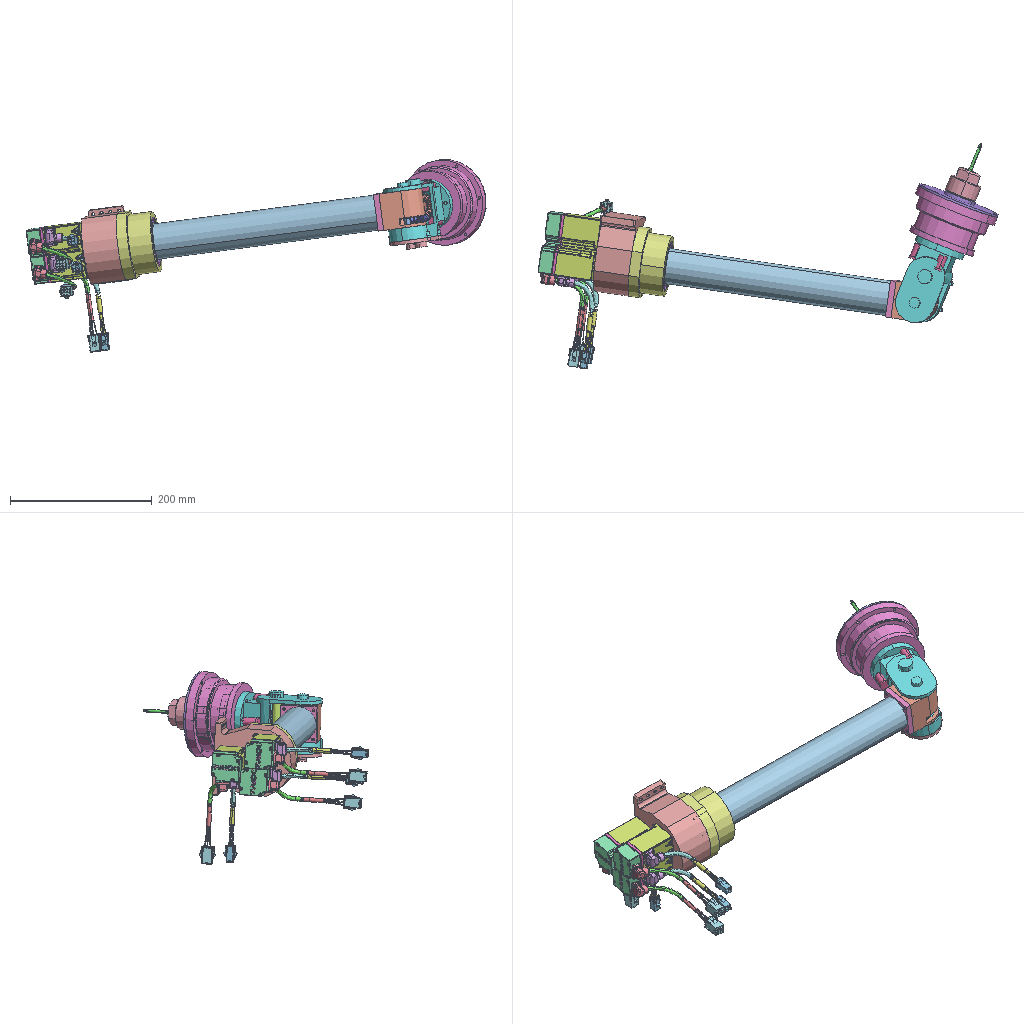Assembly | SolidWorks | 59 different items | 88 placed | box 650 x 319 x 272 mm
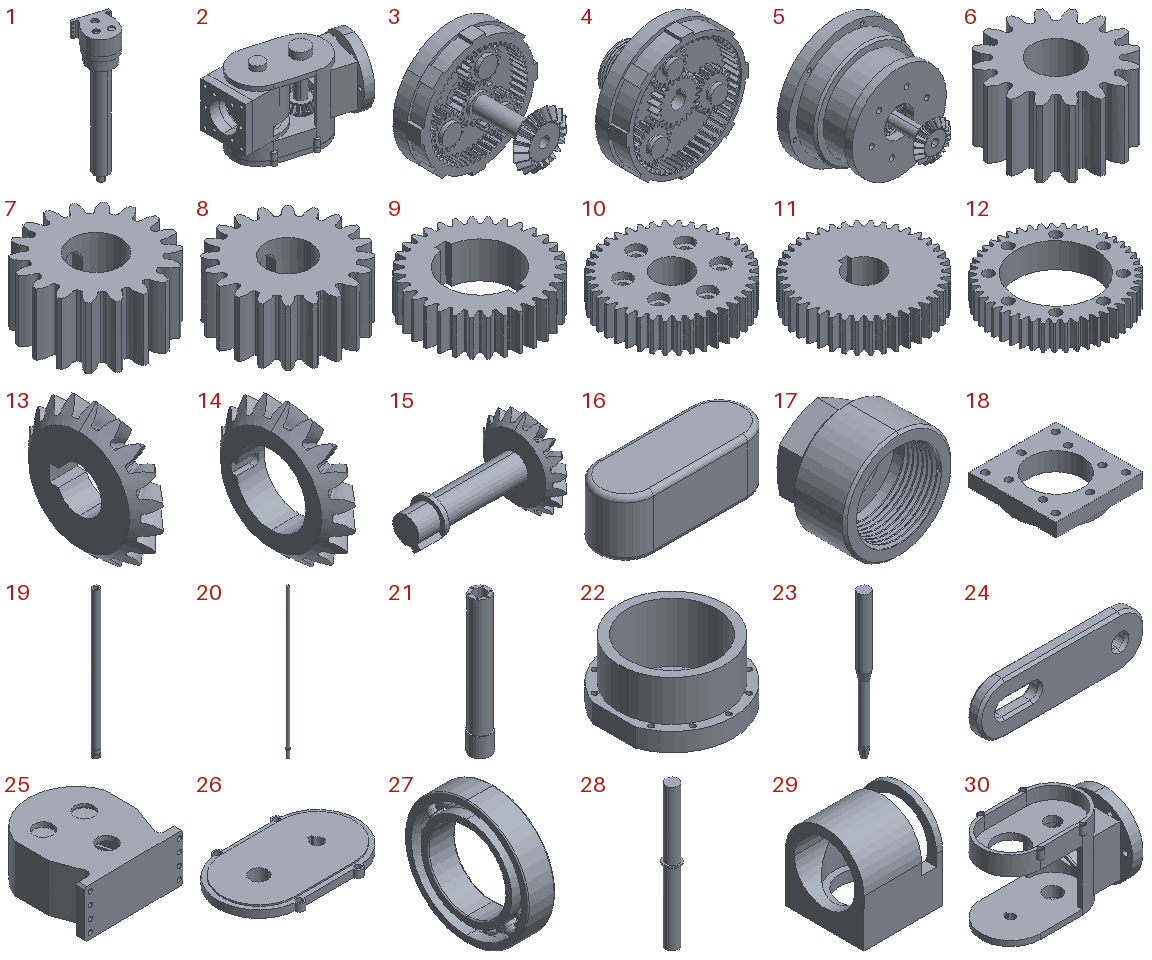Parts list (item | name | quantity | parent item | size | volume | features):
1 | (subassembly) | x1 | - | - | 966521 mm3 | features CompositeCurve 9
2 | (subassembly) | x1 | - | 136.042 x 89.867 x 96.4 mm | 262623 mm3 | features CompositeCurve 5
3 | (subassembly) | x1 | in 5 | 84 x 79.158 x 84 mm | 93250 mm3 | features CompositeCurve 17
4 | (subassembly) | x1 | in 5 | 100 x 55 x 100 mm | 136312 mm3 | features CompositeCurve 16
5 | (subassembly) | x1 | - | 121 x 130.788 x 121 mm | 395483 mm3 | features CompositeCurve 2
6 | - | x1 | - | 17.771 x 17.771 x 10 mm | 1584 mm3 | features ICE 2, CirPattern 1, Extrusion 1, RefAxis 1
7 | - | x3 | in 1 | 20 x 19.803 x 10 mm | 1962 mm3 | features ICE 3, CirPattern 1, Extrusion 1, RefAxis 1
8 | - | x1 | in 1 | 21.827 x 21.827 x 10 mm | 2548 mm3 | features ICE 3, CirPattern 1, Extrusion 1, RefAxis 1
9 | - | x1 | in 1 | 33.901 x 33.901 x 10 mm | 5034 mm3 | features ICE 3, CirPattern 1, Extrusion 1, RefAxis 1
10 | - | x1 | in 2 | 41.923 x 41.923 x 10 mm | 10682 mm3 | features ICE 4, CirPattern 1, Extrusion 1, RefAxis 1
11 | - | x1 | in 2 | 41.923 x 41.923 x 10 mm | 11284 mm3 | features ICE 3, CirPattern 1, Extrusion 1, RefAxis 1
12 | - | x1 | in 1 | 48.992 x 48.968 x 10 mm | 8395 mm3 | features ICE 3, CirPattern 1, Extrusion 1, RefAxis 1
13 | - | x2 | in 2 | 6.349 x 23.982 x 24.268 mm | 1239 mm3 | features 3DProfileFeature 12, ICE 2, BlendCut 1, CirPattern 1, RefAxis 1, Revolution 1
14 | - | x2 | in 2 | 10.158 x 38.37 x 38.828 mm | 3651 mm3 | features 3DProfileFeature 12, ICE 2, BlendCut 1, CirPattern 1, RefAxis 1, Revolution 1
15 | - | x1 | in 3 | 60.158 x 38.37 x 38.828 mm | 11848 mm3 | features 3DProfileFeature 12, ICE 2, BlendCut 1, CirPattern 1, RefAxis 1, Revolution 1
16 | - | x1 | - | 8 x 3 x 3 mm | 65.694 mm3 | features Extrusion 1, Fillet 1
17 | - | x1 | - | 46 x 37.5 x 46 mm | 24273 mm3 | features Chamfer 1, ICE 1, Revolution 1, SweepThread 1
18 | - | x1 | in 2 | 52 x 52 x 11 mm | 16978 mm3 | features ICE 4, Extrusion 1
19 | - | x1 | in 1 | 20 x 20 x 428 mm | 85566 mm3 | features ICE 11, Extrusion 1
20 | - | x1 | in 1 | 10 x 10 x 449.1 mm | 22555 mm3 | features ICE 8, Extrusion 1
21 | - | x1 | in 1 | 55 x 55 x 373 mm | 451503 mm3 | features ICE 4, Chamfer 1, Extrusion 1
22 | - | x1 | in 1 | 93.67 x 100 x 53 mm | 120948 mm3 | features ICE 4, Extrusion 1
23 | - | x1 | - | 6 x 6 x 74.531 mm | 1533 mm3 | features Revolution 2, Chamfer 1, Fillet 1, ICE 1
24 | - | x1 | - | 65.398 x 5 x 20 mm | 5328 mm3 | features Chamfer 1, Extrusion 1
25 | - | x1 | in 1 | 105 x 111.51 x 50 mm | 200027 mm3 | features ICE 10, Fillet 2, Chamfer 1, Extrusion 1
26 | - | x1 | in 2 | 96 x 62 x 14 mm | 28190 mm3 | features ICE 6, Extrusion 1
27 | - | x6 | in 1 | 7 x 32 x 32 mm | 2176 mm3 | features Revolution 5, CirPattern 2, RevCut 2
28 | - | x1 | in 2 | 10 x 10 x 89.39 mm | 4408 mm3 | features ICE 3, Extrusion 1
29 | - | x1 | in 2 | 52 x 52 x 57.532 mm | 52074 mm3 | features ICE 8, Extrusion 1
30 | - | x1 | in 2 | 118 x 72 x 83.4 mm | 115951 mm3 | features ICE 17, Cut 1, Extrusion 1
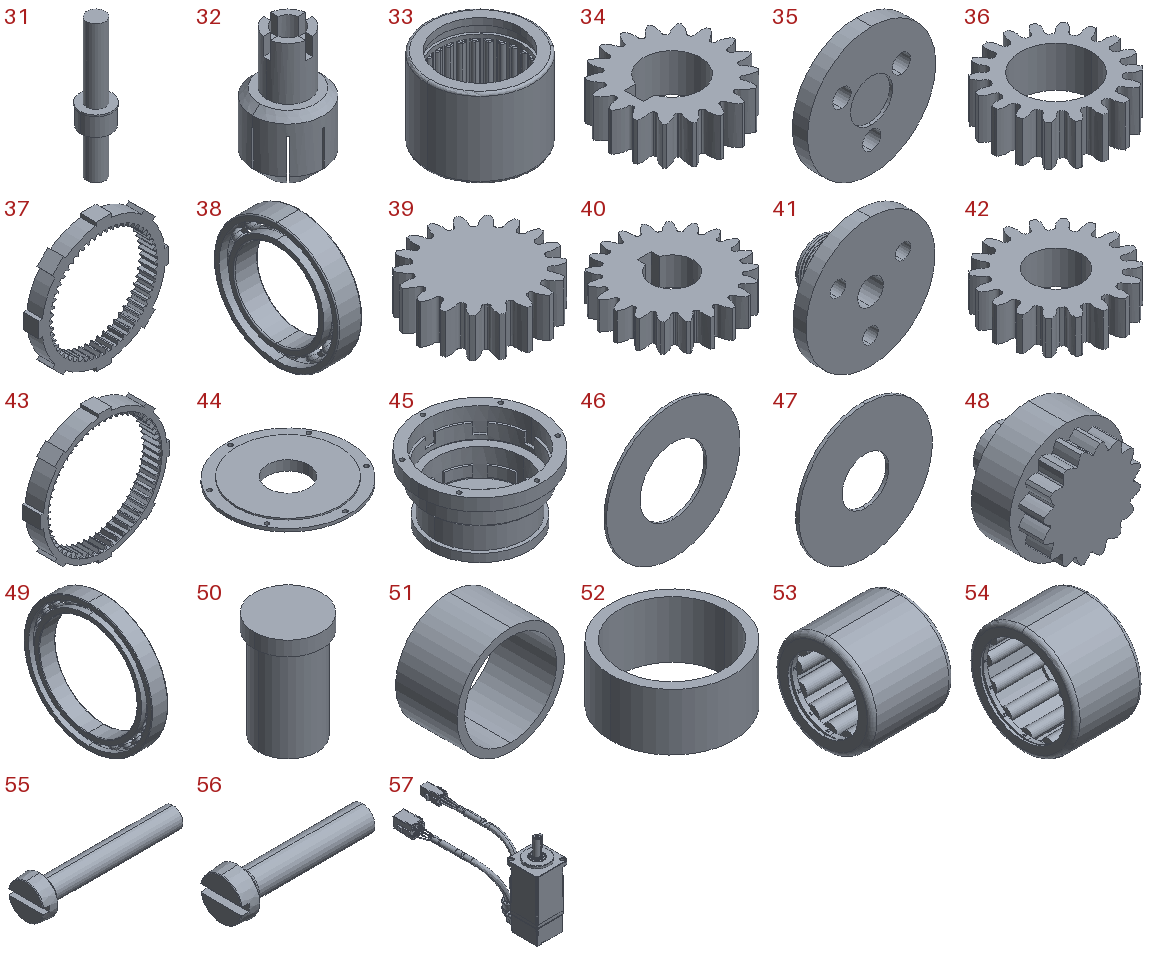31 | - | x1 | in 2 | 21 x 21 x 90.35 mm | 12865 mm3 | features ICE 4, Extrusion 1
32 | - | x1 | - | 20 x 20 x 35 mm | 5438 mm3 | features ICE 2, Chamfer 1, Revolution 1
33 | - | x1 | - | 16 x 16 x 12 mm | 801.274 mm3 | features CirPattern 2, Revolution 2, RevCut 1
34 | - | x1 | in 3 | 25.875 x 25.587 x 8 mm | 2389 mm3 | features CirPattern 1, Cut 1, Extrusion 1, ICE 1, RefAxis 1
35 | - | x1 | in 3 | 84 x 20 x 84 mm | 50141 mm3 | features ICE 3, CirPattern 1, Extrusion 1
36 | - | x3 | in 3 | 24.125 x 23.91 x 8 mm | 1615 mm3 | features ICE 2, CirPattern 1, Extrusion 1, RefAxis 1
37 | - | x1 | in 3 | 84 x 10 x 84 mm | 15215 mm3 | features CirPattern 1, Extrusion 1, ICE 1
38 | - | x1 | - | 7 x 37 x 37 mm | 2477 mm3 | features Revolution 5, CirPattern 2, RevCut 2
39 | - | x1 | - | 25 x 24.753 x 8 mm | 3124 mm3 | features CirPattern 1, Extrusion 1, ICE 1, RefAxis 1
40 | - | x1 | in 4 | 35.207 x 35.115 x 8 mm | 5449 mm3 | features CirPattern 1, Cut 1, Extrusion 1, ICE 1, RefAxis 1
41 | - | x1 | in 4 | 100 x 40 x 100 mm | 92937 mm3 | features ICE 3, Extrusion 1, SweepThread 1
42 | - | x3 | in 4 | 29.25 x 28.982 x 8 mm | 3303 mm3 | features CirPattern 1, Cut 1, Extrusion 1, ICE 1, RefAxis 1
43 | - | x1 | in 4 | 100 x 14 x 100 mm | 20184 mm3 | features CirPattern 1, Extrusion 1, ICE 1
44 | - | x1 | - | 120 x 120 x 9.5 mm | 41855 mm3 | features ICE 1, Revolution 1
45 | - | x1 | in 5 | 121 x 121 x 64.094 mm | 133004 mm3 | features ICE 4, Chamfer 1, CirPattern 1, Revolution 1
46 | - | x1 | in 5 | 100 x 2 x 100 mm | 11781 mm3 | features Extrusion 1
47 | - | x1 | in 5 | 85 x 2 x 85 mm | 9935 mm3 | features Extrusion 1
48 | - | x1 | in 5 | 30 x 25 x 30 mm | 11200 mm3 | features Cut 1, Extrusion 1, ICE 1
49 | - | x2 | in 1 | 9 x 72 x 72 mm | 10111 mm3 | features Revolution 5, CirPattern 2, RevCut 2
50 | - | x6 | in 3, 4 | 14 x 14 x 22 mm | 2611 mm3 | features Revolution 1
51 | - | x3 | in 3 | 14 x 8 x 14 mm | 326.726 mm3 | features Extrusion 1
52 | - | x1 | in 1 | 65 x 65 x 30 mm | 28274 mm3 | features Extrusion 1
53 | - | x7 | in 1 | 10 x 12 x 12 mm | 357.664 mm3 | features Revolution 3, CirPattern 2, MirrorPattern 2, Fillet 1, RevCut 1
54 | - | x1 | in 2 | 10 x 16 x 16 mm | 411.682 mm3 | features Revolution 3, CirPattern 2, MirrorPattern 2, Fillet 1, RevCut 1
55 | - | x1 | - | 22 x 5.5 x 5.5 mm | 181.48 mm3 | features Cut 1, LPattern 1, RevCut 1, Revolution 1
56 | - | x1 | - | 22.6 x 7 x 7 mm | 333.571 mm3 | features Cut 1, LPattern 1, RevCut 1, Revolution 1
57 | - | x3 | - | - | - | features BaseBody 54
58 | GB/T 301-2015[Single-Direction Thrust Ball Bearing[Type 51000]51204] | x1 | - | - | - | -
59 | Forearm Rotation Rear Flange | x1 | - | - | - | -
Mates (type | each side: item.copy, entity, surface, feature):
In the top assembly
Concentric | 21.1 face cylinder Boss-Extrude2 | 18.1 face cylinder Boss-Extrude1
Concentric | 21.1 face cylinder Cut-Extrude2 | 18.1 face cylinder Cut-Extrude1
Parallel | 20.1 face plane Cut-Extrude2 | 13.1 face plane Cut-Extrude2
Coincident | 20.1 face plane Cut-Extrude2 | 13.1 face plane Cut-Extrude2
Parallel | 19.1 face plane Cut-Extrude4 | 14.1 face plane Cut-Extrude2
Coincident | 19.1 face plane Cut-Extrude4 | 14.1 face plane Cut-Extrude2
Coincident | 21.1 face plane Boss-Extrude3 | 18.1 face plane Boss-Extrude2
Concentric | 7.1 face cylinder Cut-Extrude2 | 57.1 face cylinder Imported
Parallel | 25.1 face plane Boss-Extrude2 | 57.1 face plane Imported
Concentric | 7.2 face cylinder Cut-Extrude2 | 57.2 face cylinder Imported
Coincident | 25.1 face plane Boss-Extrude1 | 57.1 face plane Imported
Parallel | 57.1 face plane Imported | 57.2 face plane Imported
Coincident | 25.1 face plane Boss-Extrude1 | 57.2 face plane Imported
Concentric | 7.3 face cylinder Cut-Extrude2 | 57.3 face cylinder Imported
Parallel | 57.1 face plane Imported | 57.3 face plane Imported
Coincident | 25.1 face plane Boss-Extrude1 | 57.3 face plane Imported
Concentric | assembly face | 32.1 face cylinder Revolve1
Concentric | 30.1 face cylinder Boss-Extrude10 | 45.1 face cylinder Boss-Extrude1
Coincident | 14.2 select_type:25 | 15.1 select_type:25
GearDim | 15.1 select_type:24 | 14.2 select_type:24
Concentric | 41.1 face cylinder Boss-Extrude2 | 44.1 face cylinder Revolve1
Coincident | 45.1 face plane Revolve1 | 44.1 face plane Revolve1
Concentric | 45.1 face cylinder Boss-Extrude2 | 44.1 face cylinder Cut-Extrude1
Concentric | 32.1 face cylinder Revolve1 | 41.1 face cylinder Boss-Extrude1
Coincident | 32.1 face plane Cut-Extrude2 | 41.1 face plane Boss-Extrude4
Coincident | 32.1 face plane Revolve1 | 41.1 face plane Boss-Extrude3
Concentric | 32.1 face cylinder Revolve1 | 23.1 face cylinder Revolve1
Coincident | 32.1 face cone Revolve1 | 17.1 face cone Revolve1
In subassembly 2
Concentric | 29.1 face cylinder Cut-Extrude3 | 14.3 face cylinder Cut-Extrude1
Concentric | 29.1 face cylinder Cut-Extrude3 | 13.2 face cylinder Cut-Extrude1
Concentric | 29.1 face cylinder Cut-Extrude5 | 13.3 face cylinder Cut-Extrude1
Coincident | 13.3 select_type:25 | 13.2 select_type:25
GearDim | 13.2 select_type:24 | 13.3 select_type:24
Concentric | 29.1 face cylinder Cut-Extrude2 | 18.2 face cylinder Boss-Extrude1
Concentric | 29.1 face cylinder Cut-Extrude1 | 18.2 face cylinder Cut-Extrude2
Coincident | 29.1 face plane Boss-Extrude1 | 18.2 face plane Boss-Extrude2
Parallel | 29.1 face plane Boss-Extrude1 | 30.2 face plane Boss-Extrude1
DistanceDim | 30.2 face plane Boss-Extrude1 | 29.1 face plane Boss-Extrude1
Concentric | 29.1 face cylinder Cut-Extrude5 | 30.2 face cylinder Cut-Extrude1
Concentric | 29.1 face cylinder Cut-Extrude5 | 10.1 face cylinder Cut-Extrude2
DistanceDim | 10.1 face plane Boss-Extrude1 | 30.2 face plane Boss-Extrude1
Concentric | 30.2 face cylinder Cut-Extrude2 | 11.1 face cylinder Cut-Extrude2
Coincident | 10.1 face plane Boss-Extrude1 | 11.1 face plane Boss-Extrude1
GearDim | 11.1 select_type:24 | 10.1 select_type:24
Concentric | 30.2 face cylinder Cut-Extrude2 | 14.4 face cylinder Cut-Extrude1
Concentric | 30.2 face cylinder Cut-Extrude3 | 54.1 face cylinder Boss-Revolve2
Coincident | 30.2 face plane Boss-Extrude3 | 54.1 face plane Boss-Revolve2
Parallel | 11.1 face plane Cut-Extrude3 | 14.4 face plane Cut-Extrude2
Concentric | 10.1 face cylinder Cut-Extrude2 | 26.1 edge
Concentric | 11.1 face cylinder Cut-Extrude2 | 26.1 face cylinder Cut-Extrude2
Concentric | 30.2 face cylinder Cut-Extrude9 | 26.1 face cylinder Cut-Extrude1
Coincident | 30.2 face plane Boss-Extrude7 | 26.1 face plane Boss-Extrude1
Concentric | 26.1 face cylinder Cut-Extrude2 | 28.1 face cylinder Boss-Extrude1
Parallel | 26.1 face plane Cut-Extrude3 | 28.1 face plane Cut-Extrude1
Coincident | 26.1 face plane Cut-Extrude3 | 28.1 face plane Cut-Extrude1
Coincident | 26.1 face plane Cut-Extrude2 | 28.1 face plane Boss-Extrude1
Coincident | 30.2 edge | 28.1 face plane Cut-Extrude1
Parallel | 13.3 face plane Cut-Extrude2 | 28.1 face plane Cut-Extrude1
Concentric | 30.2 face cylinder Cut-Extrude2 | 31.1 face cylinder Boss-Extrude1
Parallel | 14.4 face plane Cut-Extrude2 | 31.1 face plane Cut-Extrude1
Coincident | 14.4 face plane Cut-Extrude2 | 31.1 face plane Cut-Extrude1
Coincident | 30.2 face plane Cut-Extrude3 | 31.1 face plane Boss-Extrude4
In subassembly 5
Concentric | 43.1 face cylinder Boss-Extrude1 | 5.1 face
Parallel | 35.1 face surface:4009 CirPattern3 | 48.1 face surface:4009 Boss-Extrude1
Concentric | 35.1 select_type:24 | 48.1 select_type:24
Coordinate | 3.1 select_type:25 | 5.1 select_type:11
Parallel | 3.1 plane | 5.1 plane
Coincident | 35.1 face plane Boss-Extrude6 | 48.1 face plane Boss-Extrude1
Lock | 35.1 select_type:0 | 48.1 select_type:0
Concentric | 40.1 face cylinder Cut-Extrude2 | 48.1 face cylinder Cut-Extrude1
Coincident | 40.1 face plane Cut-Extrude2 | 48.1 face plane Cut-Extrude1
Lock | 43.1 select_type:0 | 37.1 select_type:0
Parallel | 43.1 face plane Boss-Extrude1 | 37.1 face plane Boss-Extrude3
Concentric | 41.2 face cylinder Boss-Extrude1 | 45.2 face cylinder Revolve1
Concentric | 43.1 face cylinder Boss-Extrude1 | 46.1 face cylinder Boss-Extrude1
Coincident | 43.1 face plane Boss-Extrude1 | 46.1 face plane Boss-Extrude1
Coincident | 43.1 face plane Boss-Extrude1 | 45.2 face plane CirPattern5
Concentric | 45.2 face cylinder Revolve1 | 47.1 face cylinder Boss-Extrude1
Coincident | 45.2 face plane Revolve1 | 47.1 face plane Boss-Extrude1
Coincident | 45.2 face plane Revolve1 | 46.1 face plane Boss-Extrude1
In subassembly 3
Coincident | 36.1 face plane Boss-Extrude1 | 36.2 face plane Boss-Extrude1
Coincident | 34.1 face plane Boss-Extrude1 | 36.2 face plane Boss-Extrude1
Coincident | 34.1 face plane Boss-Extrude1 | 36.3 face plane Boss-Extrude1
DistanceDim | 37.2 face plane Boss-Extrude3 | 36.2 face plane Boss-Extrude1
Coordinate | 37.2 select_type:25 | 3.2 select_type:11
Parallel | 37.2 face plane Boss-Extrude3 | 3.2 plane
GearDim | 34.1 select_type:24 | 36.2 select_type:24
GearDim | 36.3 select_type:24 | 34.1 select_type:24
GearDim | 34.1 select_type:24 | 36.1 select_type:24
GearDim | 36.1 select_type:24 | 37.2 select_type:24
GearDim | 37.2 select_type:24 | 36.3 select_type:24
GearDim | 37.2 select_type:24 | 36.2 select_type:24
Concentric | 36.2 face cylinder Cut-Extrude2 | 51.1 face cylinder Boss-Extrude1
Coincident | 36.2 face plane Boss-Extrude1 | 51.1 face plane Boss-Extrude1
Concentric | 36.1 face cylinder Cut-Extrude2 | 51.2 face cylinder Boss-Extrude1
Coincident | 36.1 face plane Boss-Extrude1 | 51.2 face plane Boss-Extrude1
Concentric | 36.3 face cylinder Cut-Extrude2 | 51.3 face cylinder Boss-Extrude1
Coincident | 36.3 face plane Boss-Extrude1 | 51.3 face plane Boss-Extrude1
Concentric | 51.1 face cylinder Boss-Extrude1 | 50.1 face cylinder Revolve1
Concentric | 51.3 face cylinder Boss-Extrude1 | 50.2 face cylinder Revolve1
Concentric | 51.2 face cylinder Boss-Extrude1 | 50.3 face cylinder Revolve1
Coincident | 50.3 face plane Revolve1 | 50.1 face plane Revolve1
Coincident | 50.2 face plane Revolve1 | 50.3 face plane Revolve1
Coincident | 34.1 face plane Boss-Extrude1 | 15.2 face plane Boss-Extrude2
Coincident | 34.1 face plane Cut-Extrude2 | 15.2 face plane Boss-Extrude1
Concentric | 50.2 face cylinder Revolve1 | 35.2 face cylinder Boss-Extrude1
Concentric | 50.1 face cylinder Revolve1 | 35.2 face cylinder Boss-Extrude1
Concentric | 50.3 face cylinder Revolve1 | 35.2 face cylinder Boss-Extrude1
Concentric | 37.2 face cylinder Boss-Extrude3 | 35.2 face cylinder Boss-Extrude1
Concentric | 34.1 face cylinder Cut-Extrude2 | 15.2 face cylinder Revolve1
Coincident | 50.3 face plane Revolve1 | 35.2 face plane Boss-Extrude1
In subassembly 4
Coincident | 42.1 face plane Boss-Extrude1 | 42.2 face plane Boss-Extrude1
Coincident | 42.3 face plane Boss-Extrude1 | 42.2 face plane Boss-Extrude1
Coordinate | 43.2 select_type:25 | 4.1 select_type:11
Parallel | 43.2 face plane Boss-Extrude1 | 4.1 plane
Concentric | 41.3 face cylinder Boss-Extrude1 | 43.2 face cylinder Boss-Extrude1
Concentric | 42.2 select_type:24 | 41.3 face cylinder Boss-Extrude1
Concentric | 42.1 select_type:24 | 41.3 face cylinder Boss-Extrude1
Concentric | 42.3 select_type:24 | 41.3 edge
Concentric | 40.2 select_type:24 | 41.3 face cylinder Boss-Extrude1
Coincident | 40.2 face plane Boss-Extrude1 | 42.2 face plane Boss-Extrude1
Coincident | 40.2 face plane Boss-Extrude1 | 41.3 face plane Boss-Extrude1
GearDim | 42.3 select_type:24 | 40.2 select_type:24
GearDim | 42.2 select_type:24 | 40.2 select_type:24
GearDim | 40.2 select_type:24 | 42.1 select_type:24
GearDim | 42.1 select_type:24 | 43.2 select_type:24
Concentric | 41.3 face cylinder Boss-Extrude1 | 50.3 face cylinder Revolve1
Concentric | 41.3 face cylinder Boss-Extrude1 | 50.2 face cylinder Revolve1
Concentric | 41.3 face cylinder Boss-Extrude1 | 50.1 face cylinder Revolve1
Coincident | 50.3 face plane Revolve1 | 50.1 face plane Revolve1
Coincident | 50.2 face plane Revolve1 | 50.3 face plane Revolve1
DistanceDim | 43.2 face plane Boss-Extrude1 | 41.3 face plane Boss-Extrude1
In subassembly 1
Concentric | 25.2 face cylinder Cut-Extrude2 | 9.1 face cylinder Cut-Extrude2
Concentric | 25.2 face cylinder Cut-Extrude2 | 8.1 face cylinder Cut-Extrude2
Concentric | 25.2 face cylinder Cut-Extrude6 | 20.2 face cylinder Boss-Extrude2
Coincident | 25.2 face plane Cut-Extrude6 | 20.2 face plane Boss-Extrude2
Parallel | 8.1 face plane Cut-Extrude6 | 20.2 face plane Cut-Extrude1
Coincident | 8.1 face plane Cut-Extrude6 | 20.2 face plane Cut-Extrude1
DistanceDim | 8.1 face plane Boss-Extrude1 | 25.2 face plane Cut-Extrude2
Concentric | 25.2 face cylinder Cut-Extrude3 | 7.4 face cylinder Cut-Extrude2
Concentric | 25.2 face cylinder Cut-Extrude3 | 7.5 face cylinder Cut-Extrude2
Concentric | 25.2 face cylinder Cut-Extrude3 | 7.6 face cylinder Cut-Extrude2
Coincident | 8.1 face plane Boss-Extrude1 | 7.4 face plane Boss-Extrude1
GearDim | 8.1 select_type:24 | 7.4 select_type:24
Coincident | 9.1 face plane Boss-Extrude1 | 7.5 face plane Boss-Extrude1
GearDim | 7.5 select_type:24 | 9.1 select_type:24
Concentric | 20.2 face cylinder Boss-Extrude2 | 19.2 face cylinder Boss-Extrude1
Parallel | 9.1 face plane Cut-Extrude3 | 19.2 face plane Cut-Extrude2
Coincident | 9.1 face plane Cut-Extrude3 | 19.2 face plane Cut-Extrude2
Coincident | 9.1 face plane Boss-Extrude1 | 19.2 face plane Boss-Extrude2
Coincident | 9.1 face plane Boss-Extrude1 | 20.2 face plane Boss-Extrude4
Concentric | 20.2 face cylinder Boss-Extrude2 | 53.1 face cylinder Boss-Revolve2
Coincident | 20.2 face plane Boss-Extrude4 | 53.1 face plane Boss-Revolve2
Concentric | 19.2 face cylinder Boss-Extrude3 | 27.1 face cylinder Boss-Revolve4
Concentric | 25.2 face cylinder Cut-Extrude2 | 12.1 face cylinder Cut-Extrude2
Coincident | 19.2 face plane Boss-Extrude3 | 12.1 face plane Boss-Extrude1
Coincident | 7.6 face plane Boss-Extrude1 | 12.1 face plane Boss-Extrude1
GearDim | 12.1 select_type:24 | 7.6 select_type:24
Concentric | 27.1 face cylinder Boss-Revolve3 | 12.1 face cylinder Cut-Extrude2
DistanceDim | 27.1 face plane Boss-Revolve3 | 12.1 face plane Boss-Extrude1
Concentric | 25.2 face cylinder Cut-Extrude2 | 21.2 face cylinder Boss-Extrude1
Concentric | 25.2 face cylinder Boss-Extrude3 | 22.1 face cylinder Boss-Extrude1
Parallel | 25.2 face plane Cut-Extrude4 | 22.1 face plane Cut-Extrude1
Coincident | 25.2 face plane Boss-Extrude1 | 22.1 face plane Boss-Extrude1
Concentric | 22.1 face cylinder Boss-Extrude1 | 49.1 face cylinder Boss-Revolve4
Coincident | 22.1 face plane Boss-Extrude2 | 49.1 face plane Boss-Revolve3
Concentric | 22.1 face cylinder Boss-Extrude1 | 52.1 face cylinder Boss-Extrude1
Coincident | 49.1 face plane Boss-Revolve3 | 52.1 face plane Boss-Extrude1
Concentric | 22.1 face cylinder Boss-Extrude1 | 49.2 face cylinder Boss-Revolve3
Coincident | 52.1 face plane Boss-Extrude1 | 49.2 face plane Boss-Revolve3
Concentric | 20.2 face cylinder Boss-Extrude5 | 53.2 face cylinder Boss-Revolve2
DistanceDim | 53.2 face plane Boss-Revolve2 | 20.2 face plane Boss-Extrude4
Concentric | 53.3 face cylinder Boss-Revolve2 | 20.2 face cylinder Boss-Extrude5
DistanceDim | 53.3 face plane Boss-Revolve2 | 20.2 face plane Boss-Extrude4
Concentric | 19.2 face cylinder Boss-Extrude5 | 27.2 face cylinder Boss-Revolve4
DistanceDim | 27.2 face plane Boss-Revolve3 | 27.3 face plane Boss-Revolve3
Concentric | 19.2 face cylinder Boss-Extrude5 | 27.4 face cylinder Boss-Revolve3
DistanceDim | 27.2 face plane Boss-Revolve3 | 27.4 face plane Boss-Revolve3
Concentric | 19.2 face cylinder Boss-Extrude5 | 27.5 face cylinder Boss-Revolve4
DistanceDim | 27.5 face plane Boss-Revolve3 | 27.4 face plane Boss-Revolve3
Concentric | 19.2 face cylinder Boss-Extrude5 | 27.6 face cylinder Boss-Revolve3
DistanceDim | 27.5 face plane Boss-Revolve3 | 27.6 face plane Boss-Revolve3
Concentric | 20.2 face cylinder Boss-Extrude5 | 53.4 face cylinder Boss-Revolve2
Concentric | 20.2 face cylinder Boss-Extrude5 | 53.5 face cylinder Boss-Revolve2
Concentric | 20.2 face cylinder Boss-Extrude5 | 53.6 face cylinder Boss-Revolve2
DistanceDim | 53.4 face plane Boss-Revolve2 | 53.2 face plane Boss-Revolve2
DistanceDim | 53.5 face plane Boss-Revolve2 | 53.4 face plane Boss-Revolve2
DistanceDim | 53.5 face plane Boss-Revolve2 | 53.6 face plane Boss-Revolve2
Concentric | 20.2 face cylinder Boss-Extrude5 | 53.7 face cylinder Boss-Revolve2
DistanceDim | 53.7 face plane Boss-Revolve2 | 53.6 face plane Boss-Revolve2